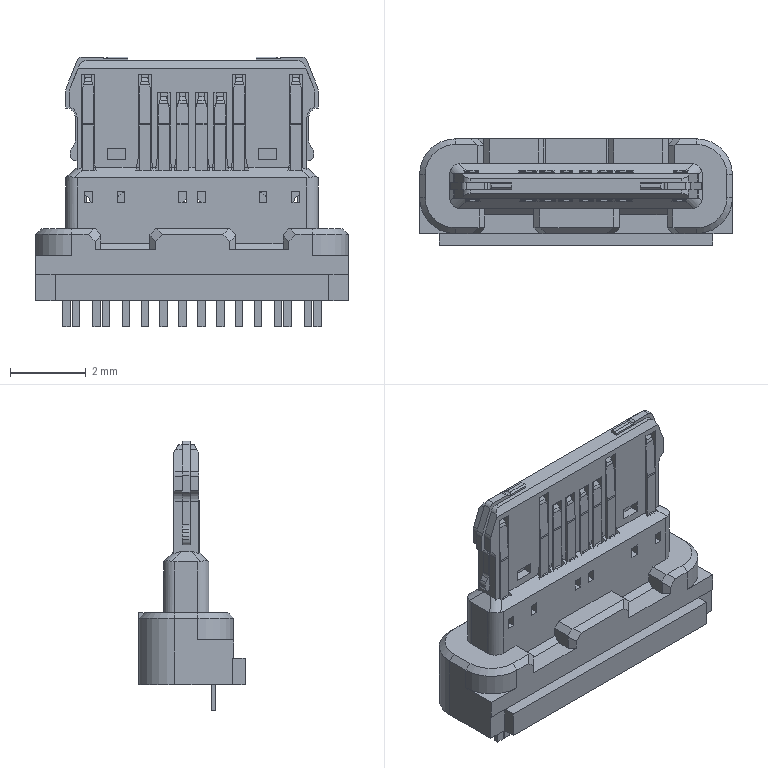Part | Creo | 1 solid | 1086 faces | box 8.29 x 2.815 x 7.15 mm | volume 54.664 mm3 | plane 934 | cylinder 148 | cone 4 | commonest cylinder face diameters 0.3 x42 0.6 x40 0.4 x24 1.6 x16 1.84 x16 1.9 x4